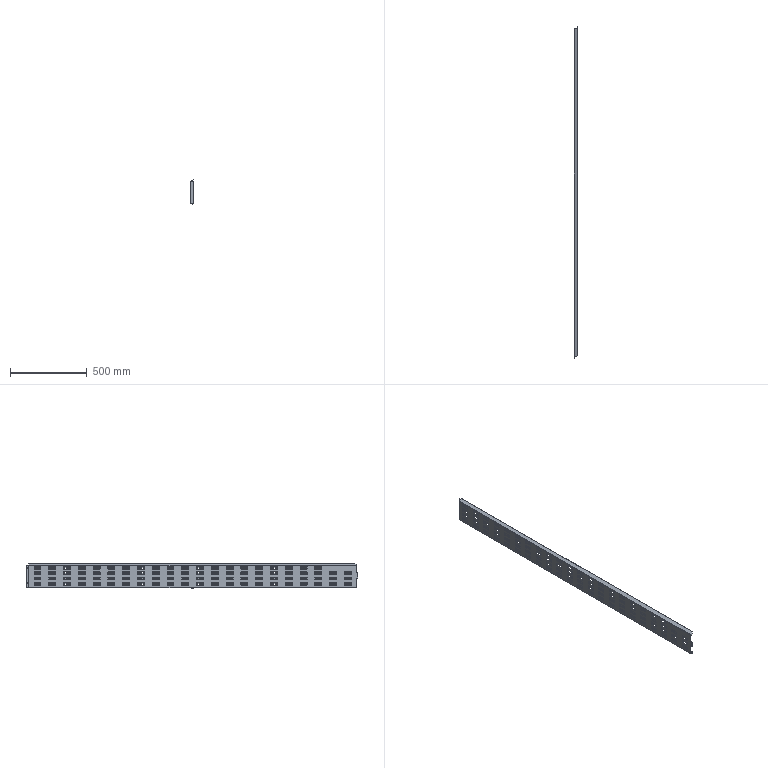Part | NX | features solid 2 | 1 solid | 3513 faces | volume 448611 mm3 | plane 2381 | cylinder 1132 | commonest cylinder face diameters 2.4 x347 4.8 x344 6 x344 6.5 x92 4 x2 1.8 x1